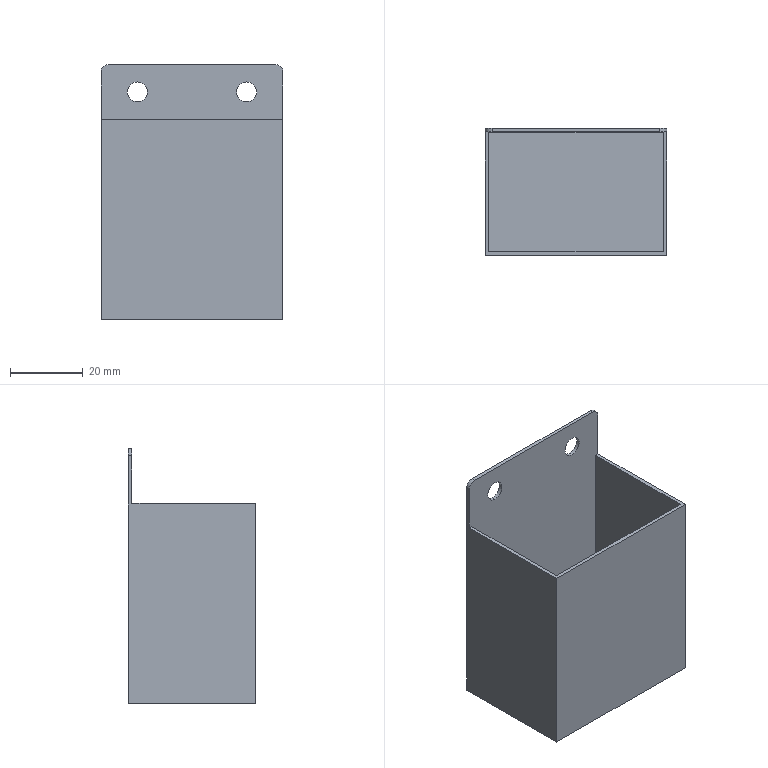Part | SolidWorks | features ICE 3, Extrusion 1, Fillet 1 | 1 solid | 18 faces | box 50 x 35 x 70 mm | volume 11415 mm3 | plane 12 | cylinder 6 | commonest cylinder face diameters 5.5 x4 4 x2
STEP:
#1=CARTESIAN_POINT('',(15.,17.5,65.25));
#2=VERTEX_POINT('',#1);
#3=CARTESIAN_POINT('',(15.,17.5,59.75));
#4=VERTEX_POINT('',#3);
#5=CARTESIAN_POINT('',(15.,17.5,62.5));
#6=DIRECTION('',(0.,-1.,0.));
#7=DIRECTION('',(0.,0.,-1.));
#8=AXIS2_PLACEMENT_3D('',#5,#6,#7);
#9=CIRCLE('',#8,2.75);
#10=EDGE_CURVE('',#2,#4,#9,.T.);
#11=ORIENTED_EDGE('',*,*,#10,.F.);
#12=CARTESIAN_POINT('',(15.,16.5,65.25));
#13=VERTEX_POINT('',#12);
#14=CARTESIAN_POINT('',(15.,28.5,65.25));
#15=DIRECTION('',(0.,-1.,0.));
#16=VECTOR('',#15,1000.);
#17=LINE('',#14,#16);
#18=EDGE_CURVE('',#2,#13,#17,.T.);
#19=ORIENTED_EDGE('',*,*,#18,.T.);
#20=CARTESIAN_POINT('',(15.,16.5,59.75));
#21=VERTEX_POINT('',#20);
#22=CARTESIAN_POINT('',(15.,16.5,62.5));
#23=DIRECTION('',(0.,-1.,0.));
#24=DIRECTION('',(0.,0.,-1.));
#25=AXIS2_PLACEMENT_3D('',#22,#23,#24);
#26=CIRCLE('',#25,2.75);
#27=EDGE_CURVE('',#13,#21,#26,.T.);
#28=ORIENTED_EDGE('',*,*,#27,.T.);
#29=CARTESIAN_POINT('',(15.,28.5,59.75));
#30=DIRECTION('',(0.,-1.,0.));
#31=VECTOR('',#30,1000.);
#32=LINE('',#29,#31);
#33=EDGE_CURVE('',#4,#21,#32,.T.);
#34=ORIENTED_EDGE('',*,*,#33,.F.);
#35=EDGE_LOOP('',(#11,#19,#28,#34));
#36=FACE_OUTER_BOUND('',#35,.T.);
#37=CARTESIAN_POINT('',(15.,28.5,62.5));
#38=DIRECTION('',(0.,-1.,0.));
#39=DIRECTION('',(0.,0.,-1.));
#40=AXIS2_PLACEMENT_3D('',#37,#38,#39);
#41=CYLINDRICAL_SURFACE('',#40,2.75);
#42=ADVANCED_FACE('',(#36),#41,.F.);
#43=CARTESIAN_POINT('',(-15.,17.5,65.25));
#44=VERTEX_POINT('',#43);
#45=CARTESIAN_POINT('',(-15.,17.5,59.75));
#46=VERTEX_POINT('',#45);
#47=CARTESIAN_POINT('',(-15.,17.5,62.5));
#48=DIRECTION('',(0.,-1.,0.));
#49=DIRECTION('',(0.,0.,-1.));
#50=AXIS2_PLACEMENT_3D('',#47,#48,#49);
#51=CIRCLE('',#50,2.75);
#52=EDGE_CURVE('',#44,#46,#51,.T.);
#53=ORIENTED_EDGE('',*,*,#52,.F.);
#54=CARTESIAN_POINT('',(-15.,16.5,65.25));
#55=VERTEX_POINT('',#54);
#56=CARTESIAN_POINT('',(-15.,28.5,65.25));
#57=DIRECTION('',(0.,-1.,0.));
#58=VECTOR('',#57,1000.);
#59=LINE('',#56,#58);
#60=EDGE_CURVE('',#44,#55,#59,.T.);
#61=ORIENTED_EDGE('',*,*,#60,.T.);
#62=CARTESIAN_POINT('',(-15.,16.5,59.75));
#63=VERTEX_POINT('',#62);
#64=CARTESIAN_POINT('',(-15.,16.5,62.5));
#65=DIRECTION('',(0.,-1.,0.));
#66=DIRECTION('',(0.,0.,-1.));
#67=AXIS2_PLACEMENT_3D('',#64,#65,#66);
#68=CIRCLE('',#67,2.75);
#69=EDGE_CURVE('',#55,#63,#68,.T.);
#70=ORIENTED_EDGE('',*,*,#69,.T.);
#71=CARTESIAN_POINT('',(-15.,28.5,59.75));
#72=DIRECTION('',(0.,-1.,0.));
#73=VECTOR('',#72,1000.);
#74=LINE('',#71,#73);
#75=EDGE_CURVE('',#46,#63,#74,.T.);
#76=ORIENTED_EDGE('',*,*,#75,.F.);
#77=EDGE_LOOP('',(#53,#61,#70,#76));
#78=FACE_OUTER_BOUND('',#77,.T.);
#79=CARTESIAN_POINT('',(-15.,28.5,62.5));
#80=DIRECTION('',(0.,-1.,0.));
#81=DIRECTION('',(0.,0.,-1.));
#82=AXIS2_PLACEMENT_3D('',#79,#80,#81);
#83=CYLINDRICAL_SURFACE('',#82,2.75);
#84=ADVANCED_FACE('',(#78),#83,.F.);
#85=CARTESIAN_POINT('',(25.,17.5,68.));
#86=VERTEX_POINT('',#85);
#87=CARTESIAN_POINT('',(25.,17.5,0.));
#88=VERTEX_POINT('',#87);
#89=CARTESIAN_POINT('',(25.,17.5,55.));
#90=DIRECTION('',(0.,0.,-1.));
#91=VECTOR('',#90,1000.);
#92=LINE('',#89,#91);
#93=EDGE_CURVE('',#86,#88,#92,.T.);
#94=ORIENTED_EDGE('',*,*,#93,.F.);
#95=CARTESIAN_POINT('',(25.,16.5,68.));
#96=VERTEX_POINT('',#95);
#97=CARTESIAN_POINT('',(25.,16.5,68.));
#98=DIRECTION('',(0.,-1.,0.));
#99=VECTOR('',#98,1000.);
#100=LINE('',#97,#99);
#101=EDGE_CURVE('',#86,#96,#100,.T.);
#102=ORIENTED_EDGE('',*,*,#101,.T.);
#103=CARTESIAN_POINT('',(25.,16.5,55.));
#104=VERTEX_POINT('',#103);
#105=CARTESIAN_POINT('',(25.,16.5,70.));
#106=DIRECTION('',(0.,0.,-1.));
#107=VECTOR('',#106,1000.);
#108=LINE('',#105,#107);
#109=EDGE_CURVE('',#96,#104,#108,.T.);
#110=ORIENTED_EDGE('',*,*,#109,.T.);
#111=CARTESIAN_POINT('',(25.,-17.5,55.));
#112=VERTEX_POINT('',#111);
#113=CARTESIAN_POINT('',(25.,17.5,55.));
#114=DIRECTION('',(0.,1.,0.));
#115=VECTOR('',#114,1000.);
#116=LINE('',#113,#115);
#117=EDGE_CURVE('',#112,#104,#116,.T.);
#118=ORIENTED_EDGE('',*,*,#117,.F.);
#119=CARTESIAN_POINT('',(25.,-17.5,0.));
#120=VERTEX_POINT('',#119);
#121=CARTESIAN_POINT('',(25.,-17.5,55.));
#122=DIRECTION('',(0.,0.,-1.));
#123=VECTOR('',#122,1000.);
#124=LINE('',#121,#123);
#125=EDGE_CURVE('',#112,#120,#124,.T.);
#126=ORIENTED_EDGE('',*,*,#125,.T.);
#127=CARTESIAN_POINT('',(25.,17.5,0.));
#128=DIRECTION('',(0.,1.,0.));
#129=VECTOR('',#128,1000.);
#130=LINE('',#127,#129);
#131=EDGE_CURVE('',#120,#88,#130,.T.);
#132=ORIENTED_EDGE('',*,*,#131,.T.);
#133=EDGE_LOOP('',(#94,#102,#110,#118,#126,#132));
#134=FACE_OUTER_BOUND('',#133,.T.);
#135=CARTESIAN_POINT('',(25.,17.5,55.));
#136=DIRECTION('',(-1.,0.,0.));
#137=DIRECTION('',(0.,-1.,0.));
#138=AXIS2_PLACEMENT_3D('',#135,#136,#137);
#139=PLANE('',#138);
#140=ADVANCED_FACE('',(#134),#139,.F.);
#141=CARTESIAN_POINT('',(15.,17.5,62.5));
#142=DIRECTION('',(0.,-1.,0.));
#143=DIRECTION('',(0.,0.,-1.));
#144=AXIS2_PLACEMENT_3D('',#141,#142,#143);
#145=CIRCLE('',#144,2.75);
#146=EDGE_CURVE('',#4,#2,#145,.T.);
#147=ORIENTED_EDGE('',*,*,#146,.T.);
#148=ORIENTED_EDGE('',*,*,#10,.T.);
#149=EDGE_LOOP('',(#147,#148));
#150=FACE_BOUND('',#149,.T.);
#151=CARTESIAN_POINT('',(-15.,17.5,62.5));
#152=DIRECTION('',(0.,-1.,0.));
#153=DIRECTION('',(0.,0.,-1.));
#154=AXIS2_PLACEMENT_3D('',#151,#152,#153);
#155=CIRCLE('',#154,2.75);
#156=EDGE_CURVE('',#46,#44,#155,.T.);
#157=ORIENTED_EDGE('',*,*,#156,.T.);
#158=ORIENTED_EDGE('',*,*,#52,.T.);
#159=EDGE_LOOP('',(#157,#158));
#160=FACE_BOUND('',#159,.T.);
#161=CARTESIAN_POINT('',(23.,17.5,70.));
#162=VERTEX_POINT('',#161);
#163=CARTESIAN_POINT('',(-23.,17.5,70.));
#164=VERTEX_POINT('',#163);
#165=CARTESIAN_POINT('',(-25.,17.5,70.));
#166=DIRECTION('',(-1.,0.,0.));
#167=VECTOR('',#166,1000.);
#168=LINE('',#165,#167);
#169=EDGE_CURVE('',#162,#164,#168,.T.);
#170=ORIENTED_EDGE('',*,*,#169,.F.);
#171=CARTESIAN_POINT('',(23.,17.5,68.));
#172=DIRECTION('',(0.,1.,0.));
#173=DIRECTION('',(0.,0.,-1.));
#174=AXIS2_PLACEMENT_3D('',#171,#172,#173);
#175=CIRCLE('',#174,2.);
#176=EDGE_CURVE('',#162,#86,#175,.T.);
#177=ORIENTED_EDGE('',*,*,#176,.T.);
#178=ORIENTED_EDGE('',*,*,#93,.T.);
#179=CARTESIAN_POINT('',(-25.,17.5,0.));
#180=VERTEX_POINT('',#179);
#181=CARTESIAN_POINT('',(-25.,17.5,0.));
#182=DIRECTION('',(-1.,0.,0.));
#183=VECTOR('',#182,1000.);
#184=LINE('',#181,#183);
#185=EDGE_CURVE('',#88,#180,#184,.T.);
#186=ORIENTED_EDGE('',*,*,#185,.T.);
#187=CARTESIAN_POINT('',(-25.,17.5,68.));
#188=VERTEX_POINT('',#187);
#189=CARTESIAN_POINT('',(-25.,17.5,55.));
#190=DIRECTION('',(0.,0.,-1.));
#191=VECTOR('',#190,1000.);
#192=LINE('',#189,#191);
#193=EDGE_CURVE('',#188,#180,#192,.T.);
#194=ORIENTED_EDGE('',*,*,#193,.F.);
#195=CARTESIAN_POINT('',(-23.,17.5,68.));
#196=DIRECTION('',(0.,1.,0.));
#197=DIRECTION('',(0.,0.,-1.));
#198=AXIS2_PLACEMENT_3D('',#195,#196,#197);
#199=CIRCLE('',#198,2.);
#200=EDGE_CURVE('',#188,#164,#199,.T.);
#201=ORIENTED_EDGE('',*,*,#200,.T.);
#202=EDGE_LOOP('',(#170,#177,#178,#186,#194,#201));
#203=FACE_OUTER_BOUND('',#202,.T.);
#204=CARTESIAN_POINT('',(-25.,17.5,55.));
#205=DIRECTION('',(0.,-1.,0.));
#206=DIRECTION('',(0.,0.,-1.));
#207=AXIS2_PLACEMENT_3D('',#204,#205,#206);
#208=PLANE('',#207);
#209=ADVANCED_FACE('',(#150,#160,#203),#208,.F.);
#210=CARTESIAN_POINT('',(-25.,16.5,68.));
#211=VERTEX_POINT('',#210);
#212=CARTESIAN_POINT('',(-25.,16.5,55.));
#213=VERTEX_POINT('',#212);
#214=CARTESIAN_POINT('',(-25.,16.5,70.));
#215=DIRECTION('',(0.,0.,-1.));
#216=VECTOR('',#215,1000.);
#217=LINE('',#214,#216);
#218=EDGE_CURVE('',#211,#213,#217,.T.);
#219=ORIENTED_EDGE('',*,*,#218,.F.);
#220=CARTESIAN_POINT('',(-25.,17.5,68.));
#221=DIRECTION('',(0.,1.,0.));
#222=VECTOR('',#221,1000.);
#223=LINE('',#220,#222);
#224=EDGE_CURVE('',#211,#188,#223,.T.);
#225=ORIENTED_EDGE('',*,*,#224,.T.);
#226=ORIENTED_EDGE('',*,*,#193,.T.);
#227=CARTESIAN_POINT('',(-25.,-17.5,0.));
#228=VERTEX_POINT('',#227);
#229=CARTESIAN_POINT('',(-25.,17.5,0.));
#230=DIRECTION('',(0.,-1.,0.));
#231=VECTOR('',#230,1000.);
#232=LINE('',#229,#231);
#233=EDGE_CURVE('',#180,#228,#232,.T.);
#234=ORIENTED_EDGE('',*,*,#233,.T.);
#235=CARTESIAN_POINT('',(-25.,-17.5,55.));
#236=VERTEX_POINT('',#235);
#237=CARTESIAN_POINT('',(-25.,-17.5,55.));
#238=DIRECTION('',(0.,0.,-1.));
#239=VECTOR('',#238,1000.);
#240=LINE('',#237,#239);
#241=EDGE_CURVE('',#236,#228,#240,.T.);
#242=ORIENTED_EDGE('',*,*,#241,.F.);
#243=CARTESIAN_POINT('',(-25.,17.5,55.));
#244=DIRECTION('',(0.,-1.,0.));
#245=VECTOR('',#244,1000.);
#246=LINE('',#243,#245);
#247=EDGE_CURVE('',#213,#236,#246,.T.);
#248=ORIENTED_EDGE('',*,*,#247,.F.);
#249=EDGE_LOOP('',(#219,#225,#226,#234,#242,#248));
#250=FACE_OUTER_BOUND('',#249,.T.);
#251=CARTESIAN_POINT('',(-25.,17.5,55.));
#252=DIRECTION('',(1.,0.,0.));
#253=DIRECTION('',(0.,0.,-1.));
#254=AXIS2_PLACEMENT_3D('',#251,#252,#253);
#255=PLANE('',#254);
#256=ADVANCED_FACE('',(#250),#255,.F.);
#257=CARTESIAN_POINT('',(-25.,-17.5,0.));
#258=DIRECTION('',(1.,0.,0.));
#259=VECTOR('',#258,1000.);
#260=LINE('',#257,#259);
#261=EDGE_CURVE('',#228,#120,#260,.T.);
#262=ORIENTED_EDGE('',*,*,#261,.T.);
#263=ORIENTED_EDGE('',*,*,#125,.F.);
#264=CARTESIAN_POINT('',(-25.,-17.5,55.));
#265=DIRECTION('',(1.,0.,0.));
#266=VECTOR('',#265,1000.);
#267=LINE('',#264,#266);
#268=EDGE_CURVE('',#236,#112,#267,.T.);
#269=ORIENTED_EDGE('',*,*,#268,.F.);
#270=ORIENTED_EDGE('',*,*,#241,.T.);
#271=EDGE_LOOP('',(#262,#263,#269,#270));
#272=FACE_OUTER_BOUND('',#271,.T.);
#273=CARTESIAN_POINT('',(-25.,-17.5,55.));
#274=DIRECTION('',(0.,1.,0.));
#275=DIRECTION('',(0.,0.,1.));
#276=AXIS2_PLACEMENT_3D('',#273,#274,#275);
#277=PLANE('',#276);
#278=ADVANCED_FACE('',(#272),#277,.F.);
#279=CARTESIAN_POINT('',(-24.,16.5,55.));
#280=VERTEX_POINT('',#279);
#281=CARTESIAN_POINT('',(-25.,16.5,55.));
#282=DIRECTION('',(1.,0.,0.));
#283=VECTOR('',#282,1000.);
#284=LINE('',#281,#283);
#285=EDGE_CURVE('',#213,#280,#284,.T.);
#286=ORIENTED_EDGE('',*,*,#285,.F.);
#287=ORIENTED_EDGE('',*,*,#247,.T.);
#288=ORIENTED_EDGE('',*,*,#268,.T.);
#289=ORIENTED_EDGE('',*,*,#117,.T.);
#290=CARTESIAN_POINT('',(24.,16.5,55.));
#291=VERTEX_POINT('',#290);
#292=CARTESIAN_POINT('',(-25.,16.5,55.));
#293=DIRECTION('',(1.,0.,0.));
#294=VECTOR('',#293,1000.);
#295=LINE('',#292,#294);
#296=EDGE_CURVE('',#291,#104,#295,.T.);
#297=ORIENTED_EDGE('',*,*,#296,.F.);
#298=CARTESIAN_POINT('',(24.,-16.5,55.));
#299=VERTEX_POINT('',#298);
#300=CARTESIAN_POINT('',(24.,16.5,55.));
#301=DIRECTION('',(0.,1.,0.));
#302=VECTOR('',#301,1000.);
#303=LINE('',#300,#302);
#304=EDGE_CURVE('',#299,#291,#303,.T.);
#305=ORIENTED_EDGE('',*,*,#304,.F.);
#306=CARTESIAN_POINT('',(-24.,-16.5,55.));
#307=VERTEX_POINT('',#306);
#308=CARTESIAN_POINT('',(24.,-16.5,55.));
#309=DIRECTION('',(1.,0.,0.));
#310=VECTOR('',#309,1000.);
#311=LINE('',#308,#310);
#312=EDGE_CURVE('',#307,#299,#311,.T.);
#313=ORIENTED_EDGE('',*,*,#312,.F.);
#314=CARTESIAN_POINT('',(-24.,16.5,55.));
#315=DIRECTION('',(0.,-1.,0.));
#316=VECTOR('',#315,1000.);
#317=LINE('',#314,#316);
#318=EDGE_CURVE('',#280,#307,#317,.T.);
#319=ORIENTED_EDGE('',*,*,#318,.F.);
#320=EDGE_LOOP('',(#286,#287,#288,#289,#297,#305,#313,#319));
#321=FACE_OUTER_BOUND('',#320,.T.);
#322=CARTESIAN_POINT('',(0.,0.,55.));
#323=DIRECTION('',(0.,0.,1.));
#324=DIRECTION('',(1.,0.,0.));
#325=AXIS2_PLACEMENT_3D('',#322,#323,#324);
#326=PLANE('',#325);
#327=ADVANCED_FACE('',(#321),#326,.T.);
#328=ORIENTED_EDGE('',*,*,#131,.F.);
#329=ORIENTED_EDGE('',*,*,#261,.F.);
#330=ORIENTED_EDGE('',*,*,#233,.F.);
#331=ORIENTED_EDGE('',*,*,#185,.F.);
#332=EDGE_LOOP('',(#328,#329,#330,#331));
#333=FACE_OUTER_BOUND('',#332,.T.);
#334=CARTESIAN_POINT('',(0.,0.,0.));
#335=DIRECTION('',(0.,0.,1.));
#336=DIRECTION('',(1.,0.,0.));
#337=AXIS2_PLACEMENT_3D('',#334,#335,#336);
#338=PLANE('',#337);
#339=ADVANCED_FACE('',(#333),#338,.F.);
#340=ORIENTED_EDGE('',*,*,#318,.T.);
#341=CARTESIAN_POINT('',(-24.,-16.5,1.));
#342=VERTEX_POINT('',#341);
#343=CARTESIAN_POINT('',(-24.,-16.5,1.));
#344=DIRECTION('',(0.,0.,1.));
#345=VECTOR('',#344,1000.);
#346=LINE('',#343,#345);
#347=EDGE_CURVE('',#342,#307,#346,.T.);
#348=ORIENTED_EDGE('',*,*,#347,.F.);
#349=CARTESIAN_POINT('',(-24.,16.5,1.));
#350=VERTEX_POINT('',#349);
#351=CARTESIAN_POINT('',(-24.,16.5,1.));
#352=DIRECTION('',(0.,-1.,0.));
#353=VECTOR('',#352,1000.);
#354=LINE('',#351,#353);
#355=EDGE_CURVE('',#350,#342,#354,.T.);
#356=ORIENTED_EDGE('',*,*,#355,.F.);
#357=CARTESIAN_POINT('',(-24.,16.5,1.));
#358=DIRECTION('',(0.,0.,1.));
#359=VECTOR('',#358,1000.);
#360=LINE('',#357,#359);
#361=EDGE_CURVE('',#350,#280,#360,.T.);
#362=ORIENTED_EDGE('',*,*,#361,.T.);
#363=EDGE_LOOP('',(#340,#348,#356,#362));
#364=FACE_OUTER_BOUND('',#363,.T.);
#365=CARTESIAN_POINT('',(-24.,16.5,1.));
#366=DIRECTION('',(-1.,0.,0.));
#367=DIRECTION('',(0.,0.,1.));
#368=AXIS2_PLACEMENT_3D('',#365,#366,#367);
#369=PLANE('',#368);
#370=ADVANCED_FACE('',(#364),#369,.F.);
#371=CARTESIAN_POINT('',(15.,16.5,62.5));
#372=DIRECTION('',(0.,-1.,0.));
#373=DIRECTION('',(0.,0.,-1.));
#374=AXIS2_PLACEMENT_3D('',#371,#372,#373);
#375=CIRCLE('',#374,2.75);
#376=EDGE_CURVE('',#21,#13,#375,.T.);
#377=ORIENTED_EDGE('',*,*,#376,.F.);
#378=ORIENTED_EDGE('',*,*,#27,.F.);
#379=EDGE_LOOP('',(#377,#378));
#380=FACE_BOUND('',#379,.T.);
#381=CARTESIAN_POINT('',(-15.,16.5,62.5));
#382=DIRECTION('',(0.,-1.,0.));
#383=DIRECTION('',(0.,0.,-1.));
#384=AXIS2_PLACEMENT_3D('',#381,#382,#383);
#385=CIRCLE('',#384,2.75);
#386=EDGE_CURVE('',#63,#55,#385,.T.);
#387=ORIENTED_EDGE('',*,*,#386,.F.);
#388=ORIENTED_EDGE('',*,*,#69,.F.);
#389=EDGE_LOOP('',(#387,#388));
#390=FACE_BOUND('',#389,.T.);
#391=ORIENTED_EDGE('',*,*,#109,.F.);
#392=CARTESIAN_POINT('',(23.,16.5,70.));
#393=VERTEX_POINT('',#392);
#394=CARTESIAN_POINT('',(23.,16.5,68.));
#395=DIRECTION('',(0.,-1.,0.));
#396=DIRECTION('',(0.,0.,1.));
#397=AXIS2_PLACEMENT_3D('',#394,#395,#396);
#398=CIRCLE('',#397,2.);
#399=EDGE_CURVE('',#96,#393,#398,.T.);
#400=ORIENTED_EDGE('',*,*,#399,.T.);
#401=CARTESIAN_POINT('',(-23.,16.5,70.));
#402=VERTEX_POINT('',#401);
#403=CARTESIAN_POINT('',(-25.,16.5,70.));
#404=DIRECTION('',(1.,0.,0.));
#405=VECTOR('',#404,1000.);
#406=LINE('',#403,#405);
#407=EDGE_CURVE('',#402,#393,#406,.T.);
#408=ORIENTED_EDGE('',*,*,#407,.F.);
#409=CARTESIAN_POINT('',(-23.,16.5,68.));
#410=DIRECTION('',(0.,-1.,0.));
#411=DIRECTION('',(0.,0.,1.));
#412=AXIS2_PLACEMENT_3D('',#409,#410,#411);
#413=CIRCLE('',#412,2.);
#414=EDGE_CURVE('',#402,#211,#413,.T.);
#415=ORIENTED_EDGE('',*,*,#414,.T.);
#416=ORIENTED_EDGE('',*,*,#218,.T.);
#417=ORIENTED_EDGE('',*,*,#285,.T.);
#418=ORIENTED_EDGE('',*,*,#361,.F.);
#419=CARTESIAN_POINT('',(24.,16.5,1.));
#420=VERTEX_POINT('',#419);
#421=CARTESIAN_POINT('',(24.,16.5,1.));
#422=DIRECTION('',(-1.,0.,0.));
#423=VECTOR('',#422,1000.);
#424=LINE('',#421,#423);
#425=EDGE_CURVE('',#420,#350,#424,.T.);
#426=ORIENTED_EDGE('',*,*,#425,.F.);
#427=CARTESIAN_POINT('',(24.,16.5,1.));
#428=DIRECTION('',(0.,0.,1.));
#429=VECTOR('',#428,1000.);
#430=LINE('',#427,#429);
#431=EDGE_CURVE('',#420,#291,#430,.T.);
#432=ORIENTED_EDGE('',*,*,#431,.T.);
#433=ORIENTED_EDGE('',*,*,#296,.T.);
#434=EDGE_LOOP('',(#391,#400,#408,#415,#416,#417,#418,#426,#432,#433));
#435=FACE_OUTER_BOUND('',#434,.T.);
#436=CARTESIAN_POINT('',(24.,16.5,1.));
#437=DIRECTION('',(0.,1.,0.));
#438=DIRECTION('',(0.,0.,1.));
#439=AXIS2_PLACEMENT_3D('',#436,#437,#438);
#440=PLANE('',#439);
#441=ADVANCED_FACE('',(#380,#390,#435),#440,.F.);
#442=ORIENTED_EDGE('',*,*,#304,.T.);
#443=ORIENTED_EDGE('',*,*,#431,.F.);
#444=CARTESIAN_POINT('',(24.,-16.5,1.));
#445=VERTEX_POINT('',#444);
#446=CARTESIAN_POINT('',(24.,16.5,1.));
#447=DIRECTION('',(0.,1.,0.));
#448=VECTOR('',#447,1000.);
#449=LINE('',#446,#448);
#450=EDGE_CURVE('',#445,#420,#449,.T.);
#451=ORIENTED_EDGE('',*,*,#450,.F.);
#452=CARTESIAN_POINT('',(24.,-16.5,1.));
#453=DIRECTION('',(0.,0.,1.));
#454=VECTOR('',#453,1000.);
#455=LINE('',#452,#454);
#456=EDGE_CURVE('',#445,#299,#455,.T.);
#457=ORIENTED_EDGE('',*,*,#456,.T.);
#458=EDGE_LOOP('',(#442,#443,#451,#457));
#459=FACE_OUTER_BOUND('',#458,.T.);
#460=CARTESIAN_POINT('',(24.,16.5,1.));
#461=DIRECTION('',(1.,0.,0.));
#462=DIRECTION('',(0.,0.,-1.));
#463=AXIS2_PLACEMENT_3D('',#460,#461,#462);
#464=PLANE('',#463);
#465=ADVANCED_FACE('',(#459),#464,.F.);
#466=ORIENTED_EDGE('',*,*,#312,.T.);
#467=ORIENTED_EDGE('',*,*,#456,.F.);
#468=CARTESIAN_POINT('',(24.,-16.5,1.));
#469=DIRECTION('',(1.,0.,0.));
#470=VECTOR('',#469,1000.);
#471=LINE('',#468,#470);
#472=EDGE_CURVE('',#342,#445,#471,.T.);
#473=ORIENTED_EDGE('',*,*,#472,.F.);
#474=ORIENTED_EDGE('',*,*,#347,.T.);
#475=EDGE_LOOP('',(#466,#467,#473,#474));
#476=FACE_OUTER_BOUND('',#475,.T.);
#477=CARTESIAN_POINT('',(24.,-16.5,1.));
#478=DIRECTION('',(0.,-1.,0.));
#479=DIRECTION('',(0.,0.,-1.));
#480=AXIS2_PLACEMENT_3D('',#477,#478,#479);
#481=PLANE('',#480);
#482=ADVANCED_FACE('',(#476),#481,.F.);
#483=ORIENTED_EDGE('',*,*,#355,.T.);
#484=ORIENTED_EDGE('',*,*,#472,.T.);
#485=ORIENTED_EDGE('',*,*,#450,.T.);
#486=ORIENTED_EDGE('',*,*,#425,.T.);
#487=EDGE_LOOP('',(#483,#484,#485,#486));
#488=FACE_OUTER_BOUND('',#487,.T.);
#489=CARTESIAN_POINT('',(0.,0.,1.));
#490=DIRECTION('',(0.,0.,-1.));
#491=DIRECTION('',(-1.,0.,0.));
#492=AXIS2_PLACEMENT_3D('',#489,#490,#491);
#493=PLANE('',#492);
#494=ADVANCED_FACE('',(#488),#493,.F.);
#495=ORIENTED_EDGE('',*,*,#407,.T.);
#496=CARTESIAN_POINT('',(23.,17.5,70.));
#497=DIRECTION('',(0.,1.,0.));
#498=VECTOR('',#497,1000.);
#499=LINE('',#496,#498);
#500=EDGE_CURVE('',#393,#162,#499,.T.);
#501=ORIENTED_EDGE('',*,*,#500,.T.);
#502=ORIENTED_EDGE('',*,*,#169,.T.);
#503=CARTESIAN_POINT('',(-23.,16.5,70.));
#504=DIRECTION('',(0.,-1.,0.));
#505=VECTOR('',#504,1000.);
#506=LINE('',#503,#505);
#507=EDGE_CURVE('',#164,#402,#506,.T.);
#508=ORIENTED_EDGE('',*,*,#507,.T.);
#509=EDGE_LOOP('',(#495,#501,#502,#508));
#510=FACE_OUTER_BOUND('',#509,.T.);
#511=CARTESIAN_POINT('',(0.,0.,70.));
#512=DIRECTION('',(0.,0.,1.));
#513=DIRECTION('',(1.,0.,0.));
#514=AXIS2_PLACEMENT_3D('',#511,#512,#513);
#515=PLANE('',#514);
#516=ADVANCED_FACE('',(#510),#515,.T.);
#517=ORIENTED_EDGE('',*,*,#60,.F.);
#518=ORIENTED_EDGE('',*,*,#156,.F.);
#519=ORIENTED_EDGE('',*,*,#75,.T.);
#520=ORIENTED_EDGE('',*,*,#386,.T.);
#521=EDGE_LOOP('',(#517,#518,#519,#520));
#522=FACE_OUTER_BOUND('',#521,.T.);
#523=CARTESIAN_POINT('',(-15.,28.5,62.5));
#524=DIRECTION('',(0.,-1.,0.));
#525=DIRECTION('',(0.,0.,-1.));
#526=AXIS2_PLACEMENT_3D('',#523,#524,#525);
#527=CYLINDRICAL_SURFACE('',#526,2.75);
#528=ADVANCED_FACE('',(#522),#527,.F.);
#529=ORIENTED_EDGE('',*,*,#18,.F.);
#530=ORIENTED_EDGE('',*,*,#146,.F.);
#531=ORIENTED_EDGE('',*,*,#33,.T.);
#532=ORIENTED_EDGE('',*,*,#376,.T.);
#533=EDGE_LOOP('',(#529,#530,#531,#532));
#534=FACE_OUTER_BOUND('',#533,.T.);
#535=CARTESIAN_POINT('',(15.,28.5,62.5));
#536=DIRECTION('',(0.,-1.,0.));
#537=DIRECTION('',(0.,0.,-1.));
#538=AXIS2_PLACEMENT_3D('',#535,#536,#537);
#539=CYLINDRICAL_SURFACE('',#538,2.75);
#540=ADVANCED_FACE('',(#534),#539,.F.);
#541=ORIENTED_EDGE('',*,*,#399,.F.);
#542=ORIENTED_EDGE('',*,*,#101,.F.);
#543=ORIENTED_EDGE('',*,*,#176,.F.);
#544=ORIENTED_EDGE('',*,*,#500,.F.);
#545=EDGE_LOOP('',(#541,#542,#543,#544));
#546=FACE_OUTER_BOUND('',#545,.T.);
#547=CARTESIAN_POINT('',(23.,0.,68.));
#548=DIRECTION('',(0.,-1.,0.));
#549=DIRECTION('',(1.,0.,0.));
#550=AXIS2_PLACEMENT_3D('',#547,#548,#549);
#551=CYLINDRICAL_SURFACE('',#550,2.);
#552=ADVANCED_FACE('',(#546),#551,.T.);
#553=ORIENTED_EDGE('',*,*,#200,.F.);
#554=ORIENTED_EDGE('',*,*,#224,.F.);
#555=ORIENTED_EDGE('',*,*,#414,.F.);
#556=ORIENTED_EDGE('',*,*,#507,.F.);
#557=EDGE_LOOP('',(#553,#554,#555,#556));
#558=FACE_OUTER_BOUND('',#557,.T.);
#559=CARTESIAN_POINT('',(-23.,0.,68.));
#560=DIRECTION('',(0.,1.,0.));
#561=DIRECTION('',(0.,0.,1.));
#562=AXIS2_PLACEMENT_3D('',#559,#560,#561);
#563=CYLINDRICAL_SURFACE('',#562,2.);
#564=ADVANCED_FACE('',(#558),#563,.T.);
#565=CLOSED_SHELL('',(#42,#84,#140,#209,#256,#278,#327,#339,#370,#441,#465,#482,#494,#516,#528,#540,#552,#564));
#566=MANIFOLD_SOLID_BREP('',#565);
#567=CARTESIAN_POINT('',(0.,0.,0.));
#568=DIRECTION('',(0.,0.,1.));
#569=DIRECTION('',(1.,0.,0.));
#570=AXIS2_PLACEMENT_3D('',#567,#568,#569);
#571=(LENGTH_UNIT()NAMED_UNIT(*)SI_UNIT(.MILLI.,.METRE.));
#572=UNCERTAINTY_MEASURE_WITH_UNIT(LENGTH_MEASURE(0.00001),#571,'','');
#573=(NAMED_UNIT(*)PLANE_ANGLE_UNIT()SI_UNIT($,.RADIAN.));
#574=(NAMED_UNIT(*)SI_UNIT($,.STERADIAN.)SOLID_ANGLE_UNIT());
#575=(GEOMETRIC_REPRESENTATION_CONTEXT(3)GLOBAL_UNCERTAINTY_ASSIGNED_CONTEXT((#572))GLOBAL_UNIT_ASSIGNED_CONTEXT((#571,#573,#574))REPRESENTATION_CONTEXT('',''));
#576=ADVANCED_BREP_SHAPE_REPRESENTATION('',(#566,#570),#575);